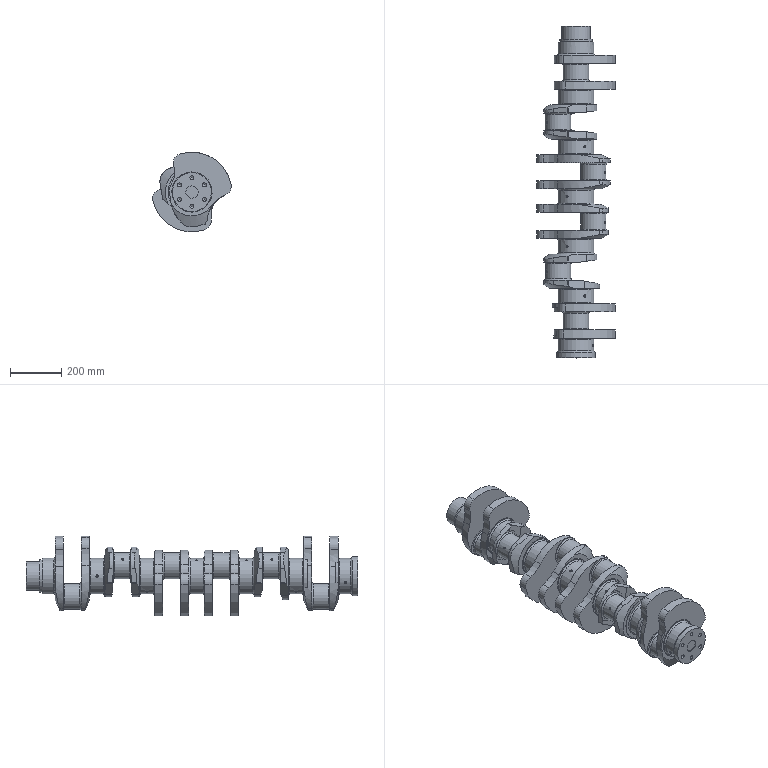Part | NX | features DATUM_CSYS 74, SKETCH 73, EXTRUDE 53, DATUM_PLANE 19, HOLE PACKAGE 19, SIMPLE HOLE 18, INTERSECTION_CURVES 13, SYMBOLIC_THREAD 12, Instance Feature 10, SKIN 10, SUBTRACT 10, UNITE 9, MIRROR 8, EXTRACT_FACE 6, EXTRACT_STRING 6, MIRROR_SET 3, BLEND 2, CHAMFER 2, Pattern Feature 2, CSUNK_HOLE 1, MOVE_OBJECT 1, SWP104 1 | 2 solids | 331 faces | box 306.35 x 1294 x 311.16 mm | volume 25921208 mm3 | cylinder 177 | plane 80 | spline 32 | torus 25 | cone 17 | commonest cylinder face diameters 10 x20 60 x16 72 x16 200 x12 294 x12 126 x10